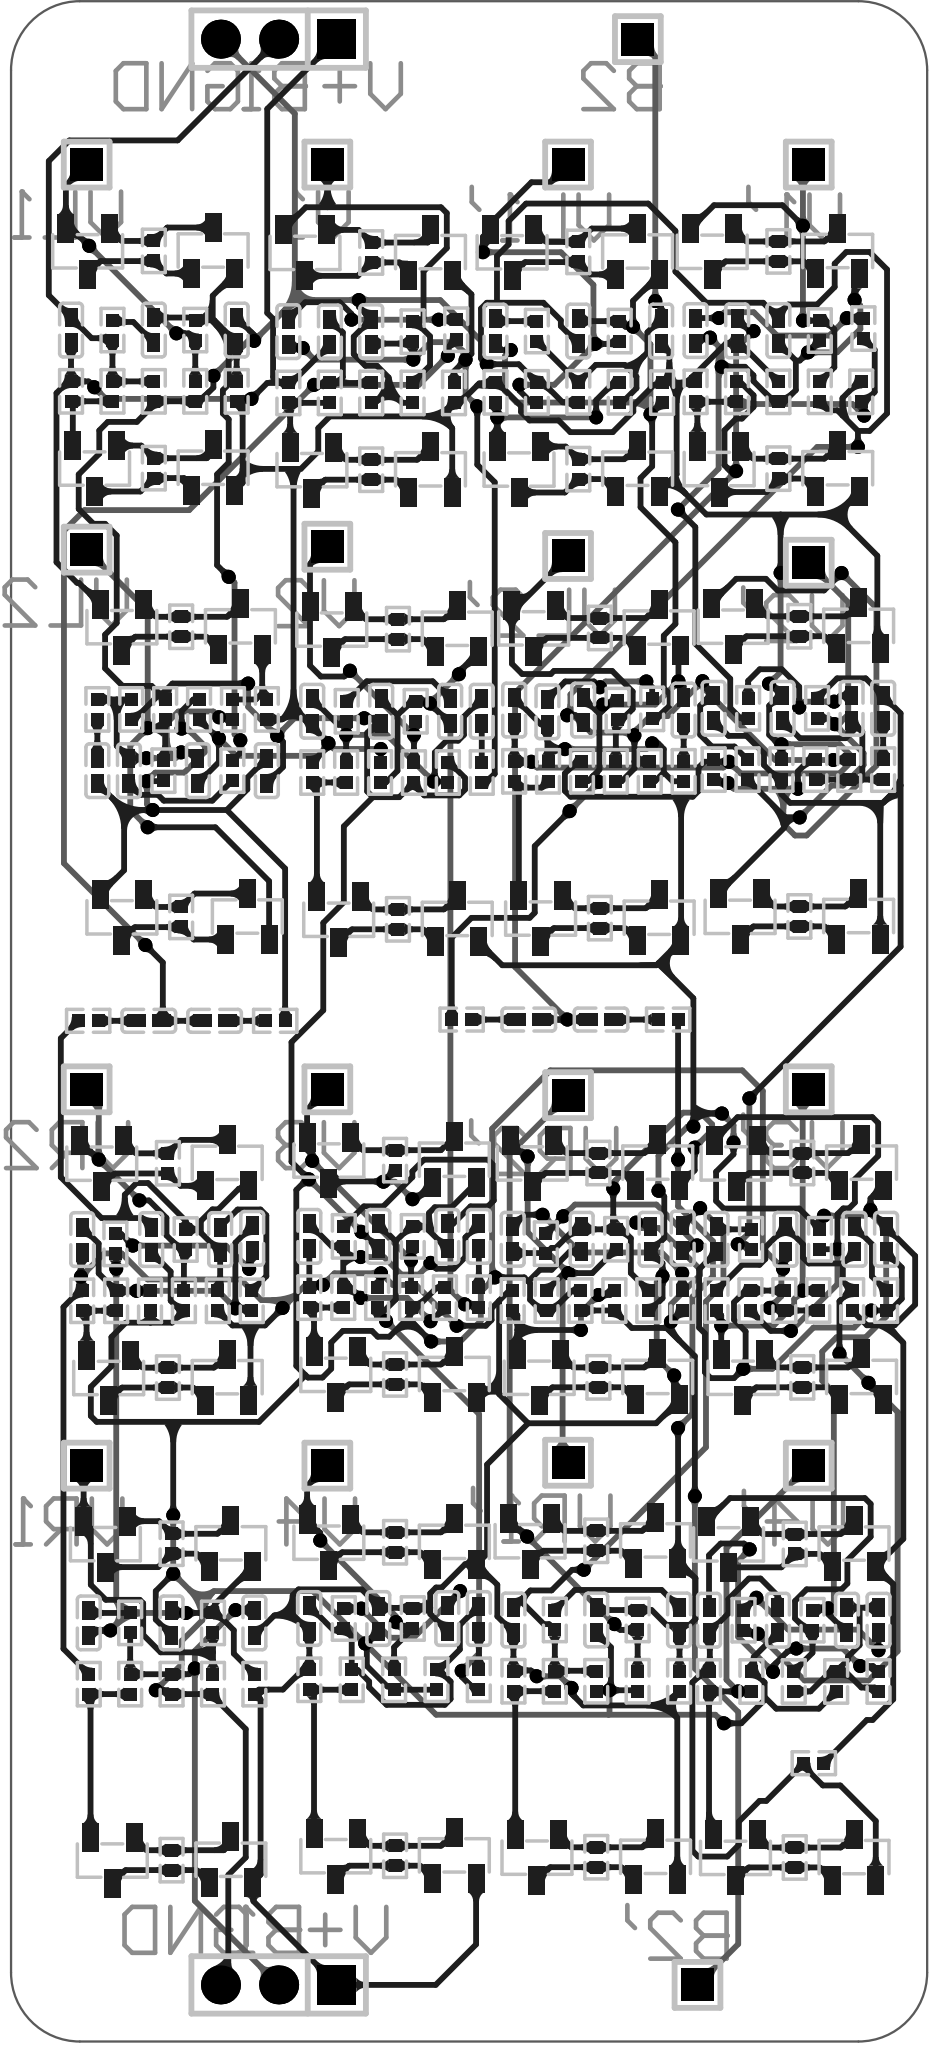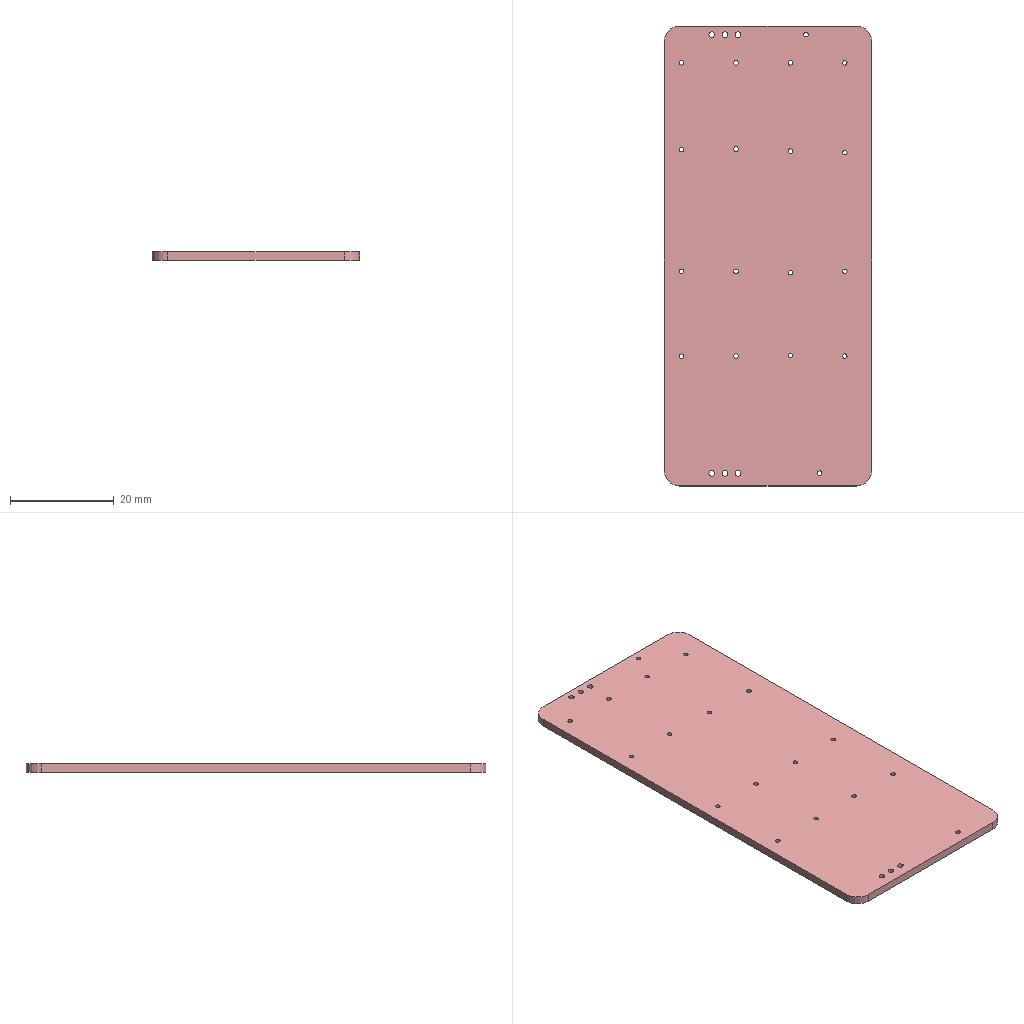Circuit board layout | Altium Designer | box 40 x 88.8 x 1.6 mm
Layer stack:
# Altium Designer layer stack of  (unit mm; dielectric type: 0 none, 1 core, 2 prepreg, 3 surface material)
index,name,kind,layer,copper_thickness_mm,dielectric_type,dielectric_thickness_mm,dielectric_material,dielectric_constant
0,Top Paste Mask Layer,other,,,,,,
1,Top Silkscreen Layer,other,,,,,,
2,Top Solder Mask Layer,dielectric,,,3,0.01,,3.3
3,Top Layer,copper,Top Layer,0.035,,,,
4,Dielectric1,dielectric,,,3,1.51,FR4,4.5
5,Bottom Layer,copper,Bottom Layer,0.035,,,,
6,Bottom Solder Mask Layer,dielectric,,,3,0.01,,3.3
7,Bottom Silkscreen Layer,other,,,,,,
8,Bottom Paste Mask Layer,other,,,,,,
# drill layer pairs: low layer,high layer
drill_pair,Top Layer,Bottom Layer
Part placement:
Designator,Comment,Layer,Footprint,Center-X(mm),Center-Y(mm),Rotation
C2,0.1uF,TopLayer,C0402,82.435,150.707,270
C4,0.1uF,TopLayer,C0402,78.819,150.707,90
C5,0.1uF,TopLayer,C0402,86.051,150.707,90
Q1,MMBT3906,TopLayer,SOT-23-3_L2.9-W1.3-P1.90-LS2.4-BR,85.023,154.171,270
Q2,MMBT3904,TopLayer,SOT-23-3_L2.9-W1.3-P1.90-LS2.4-BR,79.847,144.678,90
Q3,MMBT3906,TopLayer,SOT-23-3_L2.9-W1.3-P1.90-LS2.4-BR,85.023,144.713,270
Q4,MMBT3904,TopLayer,SOT-23-3_L2.9-W1.3-P1.90-LS2.4-BR,79.544,154.136,90
R1,1,TopLayer,R0402,80.627,150.707,270
R3,2.2K,TopLayer,R0402,82.435,148.04,270
R4,2.2K,TopLayer,R0402,86.051,148.04,90
Rb1,1K,TopLayer,R0402,82.435,144.696,270
Rb2,1K,TopLayer,R0402,82.435,154.153,270
Rp1,200K,TopLayer,R0402,78.819,148.04,270
Rp2,200K,TopLayer,R0402,84.243,150.707,270
Rs1,200,TopLayer,R0402,80.627,148.04,90
Rs2,200,TopLayer,R0402,84.243,148.04,270
Rb3,1K,TopLayer,R0402,83.627,137.791,90
Q6,MMBT3906,TopLayer,SOT-23-3_L2.9-W1.3-P1.90-LS2.4-BR,81.039,137.773,90
Q5,MMBT3904,TopLayer,SOT-23-3_L2.9-W1.3-P1.90-LS2.4-BR,86.215,137.808,270
R7,2.2K,TopLayer,R0402,81.448,134.193,270
Rp3,200K,TopLayer,R0402,87.37,134.193,90
Rs3,200,TopLayer,R0402,85.889,134.193,270
R9,2.2K,TopLayer,R0402,84.409,134.193,90
Rs4,200,TopLayer,R0402,82.929,134.193,90
C1,0.1uF,TopLayer,C0402,81.347,131.526,270
C6,0.1uF,TopLayer,C0402,84.358,131.526,90
Rp4,200K,TopLayer,R0402,82.852,131.526,90
R5,1,TopLayer,R0402,85.864,131.526,90
C7,0.1uF,TopLayer,C0402,87.37,131.526,270
Q7,MMBT3904,TopLayer,SOT-23-3_L2.9-W1.3-P1.90-LS2.4-BR,86.517,125.176,270
Rb4,1K,TopLayer,R0402,83.627,125.158,90
Q8,MMBT3906,TopLayer,SOT-23-3_L2.9-W1.3-P1.90-LS2.4-BR,81.039,125.141,90
C8,0.1uF,TopLayer,C0402,79.968,131.526,90
H1,,TopLayer,HDR-TH_3P-P2.54-V-M,87.884,163.373,180
C9,0.02uF,TopLayer,C0402,85.087,120.635,0
C17,0.02uF,TopLayer,C0402,82.215,120.635,180
R6,1,TopLayer,R0402,79.968,134.193,90
R10,1,TopLayer,R0402,87.734,120.635,0
R18,1,TopLayer,R0402,79.568,120.635,180
Rp7,200K,TopLayer,R0402,79.307,108.447,270
Rs7,200,TopLayer,R0402,80.787,108.447,90
R16,2.2K,TopLayer,R0402,82.268,108.447,270
Rs8,200,TopLayer,R0402,83.748,108.447,270
R17,2.2K,TopLayer,R0402,85.228,108.447,90
R15,1,TopLayer,R0402,86.709,108.447,270
C14,0.1uF,TopLayer,C0402,79.307,111.114,90
R19,1,TopLayer,R0402,95.635,150.725,270
C15,0.1uF,TopLayer,C0402,82.319,111.114,270
Rp8,200K,TopLayer,R0402,83.824,111.114,270
C16,0.1uF,TopLayer,C0402,85.33,111.114,90
C18,0.1uF,TopLayer,C0402,90.123,150.626,90
Rb7,1K,TopLayer,R0402,83.05,105.103,270
Q13,MMBT3904,TopLayer,SOT-23-3_L2.9-W1.3-P1.90-LS2.4-BR,80.462,105.085,90
Q14,MMBT3906,TopLayer,SOT-23-3_L2.9-W1.3-P1.90-LS2.4-BR,85.638,105.121,270
Q16,MMBT3906,TopLayer,SOT-23-3_L2.9-W1.3-P1.90-LS2.4-BR,85.638,114.451,270
Q15,MMBT3904,TopLayer,SOT-23-3_L2.9-W1.3-P1.90-LS2.4-BR,80.159,114.416,90
Rb8,1K,TopLayer,R0402,83.05,114.434,270
Rb5,1K,TopLayer,R0402,83.209,84.095,270
Q10,MMBT3906,TopLayer,SOT-23-3_L2.9-W1.3-P1.90-LS2.4-BR,85.797,84.113,270
Q9,MMBT3904,TopLayer,SOT-23-3_L2.9-W1.3-P1.90-LS2.4-BR,80.621,84.078,90
R13,2.2K,TopLayer,R0402,86.825,91.757,90
Rp5,200K,TopLayer,R0402,79.593,91.757,270
Rs5,200,TopLayer,R0402,81.401,91.757,90
R14,2.2K,TopLayer,R0402,83.209,91.757,270
Rs6,200,TopLayer,R0402,85.017,91.757,270
Rp6,200K,TopLayer,R0402,85.017,94.424,270
R11,1,TopLayer,R0402,81.401,94.424,270
C10,0.1uF,TopLayer,C0402,86.825,94.424,90
C11,0.1uF,TopLayer,C0402,83.209,94.424,270
C12,0.1uF,TopLayer,C0402,79.593,94.424,90
Q11,MMBT3904,TopLayer,SOT-23-3_L2.9-W1.3-P1.90-LS2.4-BR,80.319,97.853,90
Rb6,1K,TopLayer,R0402,83.209,97.871,270
Q12,MMBT3906,TopLayer,SOT-23-3_L2.9-W1.3-P1.90-LS2.4-BR,85.797,97.888,270
Rb9,1K,TopLayer,R0402,91.925,144.627,270
Q18,MMBT3906,TopLayer,SOT-23-3_L2.9-W1.3-P1.90-LS2.4-BR,94.513,144.644,270
Q17,MMBT3904,TopLayer,SOT-23-3_L2.9-W1.3-P1.90-LS2.4-BR,89.337,144.609,90
R20,2.2K,TopLayer,R0402,95.541,147.971,90
Rp9,200K,TopLayer,R0402,88.309,147.971,270
Rs9,200,TopLayer,R0402,90.117,147.971,90
R21,2.55K,TopLayer,R0402,91.925,147.971,270
Rs10,200,TopLayer,R0402,93.733,147.971,270
Rp10,200K,TopLayer,R0402,93.733,150.638,90
R12,1,TopLayer,R0402,80.756,110.924,270
C13,0.1uF,TopLayer,C0402,86.73,111.165,270
C19,0.1uF,TopLayer,C0402,91.925,150.638,90
C20,0.1uF,TopLayer,C0402,88.309,150.638,90
Q19,MMBT3904,TopLayer,SOT-23-3_L2.9-W1.3-P1.90-LS2.4-BR,89.034,154.067,90
Rb10,1K,TopLayer,R0402,91.925,154.084,270
Q20,MMBT3906,TopLayer,SOT-23-3_L2.9-W1.3-P1.90-LS2.4-BR,94.513,154.102,270
Rb11,1K,TopLayer,R0402,93.094,125.053,270
Q21,MMBT3904,TopLayer,SOT-23-3_L2.9-W1.3-P1.90-LS2.4-BR,90.505,125.035,90
Q22,MMBT3906,TopLayer,SOT-23-3_L2.9-W1.3-P1.90-LS2.4-BR,95.682,125.07,270
Rs11,200,TopLayer,R0402,90.831,131.445,90
R24,2.2K,TopLayer,R0402,95.272,131.445,90
R22,1,TopLayer,R0402,96.752,131.445,270
Rp11,200K,TopLayer,R0402,89.351,131.445,270
Rs12,200,TopLayer,R0402,93.792,131.445,270
R25,2.2K,TopLayer,R0402,92.312,131.445,270
C21,0.1uF,TopLayer,C0402,96.752,134.112,270
C22,0.1uF,TopLayer,C0402,89.351,134.112,90
R23,1,TopLayer,R0402,90.857,134.112,270
C23,0.1uF,TopLayer,C0402,92.362,134.112,270
C24,0.1uF,TopLayer,C0402,95.374,134.112,90
Rp12,200K,TopLayer,R0402,93.868,134.112,270
Rb12,1K,TopLayer,R0402,93.094,137.685,270
Q23,MMBT3904,TopLayer,SOT-23-3_L2.9-W1.3-P1.90-LS2.4-BR,90.203,137.668,90
Q24,MMBT3906,TopLayer,SOT-23-3_L2.9-W1.3-P1.90-LS2.4-BR,95.682,137.703,270
Rb13,1K,TopLayer,R0402,92.967,105.241,270
Q25,MMBT3904,TopLayer,SOT-23-3_L2.9-W1.3-P1.90-LS2.4-BR,90.379,105.223,90
Q26,MMBT3906,TopLayer,SOT-23-3_L2.9-W1.3-P1.90-LS2.4-BR,95.555,105.258,270
Rs13,200,TopLayer,R0402,90.704,108.585,90
R28,2.2K,TopLayer,R0402,95.145,108.585,90
R26,1,TopLayer,R0402,96.626,108.585,270
Rp13,200K,TopLayer,R0402,89.224,108.585,270
Rs14,200,TopLayer,R0402,93.665,108.585,270
R29,2.2K,TopLayer,R0402,92.185,108.585,270
C25,0.1uF,TopLayer,C0402,96.626,111.252,270
C26,0.1uF,TopLayer,C0402,89.224,111.252,90
R27,1,TopLayer,R0402,90.73,111.252,270
C27,0.1uF,TopLayer,C0402,92.235,111.252,270
C28,0.1uF,TopLayer,C0402,95.247,111.252,90
Rp14,200K,TopLayer,R0402,93.741,111.252,270
Rb14,1K,TopLayer,R0402,92.967,114.571,270
Q27,MMBT3904,TopLayer,SOT-23-3_L2.9-W1.3-P1.90-LS2.4-BR,90.076,114.554,90
Q28,MMBT3906,TopLayer,SOT-23-3_L2.9-W1.3-P1.90-LS2.4-BR,95.555,114.589,270
Rb15,1K,TopLayer,R0402,92.967,84.286,270
Q29,MMBT3904,TopLayer,SOT-23-3_L2.9-W1.3-P1.90-LS2.4-BR,90.379,84.268,90
Q30,MMBT3906,TopLayer,SOT-23-3_L2.9-W1.3-P1.90-LS2.4-BR,95.555,84.303,270
Rs15,200,TopLayer,R0402,91.074,91.948,90
R32,2.2K,TopLayer,R0402,94.775,91.948,270
R30,1,TopLayer,R0402,96.626,91.948,270
Rp15,200K,TopLayer,R0402,89.224,91.948,270
Rs16,200,TopLayer,R0402,92.925,91.948,270
R35,2.2K,TopLayer,R0402,104.626,147.984,270
C29,0.1uF,TopLayer,C0402,96.626,94.615,270
C30,0.1uF,TopLayer,C0402,89.224,94.615,90
R31,1,TopLayer,R0402,90.73,94.615,270
C31,0.1uF,TopLayer,C0402,92.235,94.615,270
C32,0.1uF,TopLayer,C0402,95.247,94.615,90
Rp16,200K,TopLayer,R0402,93.741,94.615,270
Rb16,1K,TopLayer,R0402,92.967,97.934,270
Q31,MMBT3904,TopLayer,SOT-23-3_L2.9-W1.3-P1.90-LS2.4-BR,90.076,97.917,90
Q32,MMBT3906,TopLayer,SOT-23-3_L2.9-W1.3-P1.90-LS2.4-BR,95.555,97.952,270
Q33,MMBT3904,TopLayer,SOT-23-3_L2.9-W1.3-P1.90-LS2.4-BR,98.379,144.635,90
Q34,MMBT3906,TopLayer,SOT-23-3_L2.9-W1.3-P1.90-LS2.4-BR,103.556,144.67,270
Rb17,1K,TopLayer,R0402,100.968,144.653,270
R36,2.2K,TopLayer,R0402,100.968,147.997,270
Rs17,200,TopLayer,R0402,102.776,147.997,270
Rp17,200K,TopLayer,R0402,97.352,147.997,270
Rs18,200,TopLayer,R0402,99.16,147.997,90
Rp18,200K,TopLayer,R0402,102.776,150.664,270
R33,1,TopLayer,R0402,99.16,150.664,270
C33,0.1uF,TopLayer,C0402,104.584,150.664,90
C34,0.1uF,TopLayer,C0402,100.968,150.664,270
C35,0.1uF,TopLayer,C0402,97.352,150.664,90
Q36,MMBT3906,TopLayer,SOT-23-3_L2.9-W1.3-P1.90-LS2.4-BR,103.556,154.128,270
Rb18,1K,TopLayer,R0402,100.968,154.11,270
Q35,MMBT3904,TopLayer,SOT-23-3_L2.9-W1.3-P1.90-LS2.4-BR,98.077,154.093,90
Rb19,1K,TopLayer,R0402,101.909,125.106,270
Q37,MMBT3904,TopLayer,SOT-23-3_L2.9-W1.3-P1.90-LS2.4-BR,99.321,125.088,90
Q38,MMBT3906,TopLayer,SOT-23-3_L2.9-W1.3-P1.90-LS2.4-BR,104.498,125.123,270
R34,1,TopLayer,R0402,104.193,134.216,270
C36,0.1uF,TopLayer,C0402,99.621,134.089,90
R38,2.2K,TopLayer,R0402,104.088,131.498,90
Rs19,200,TopLayer,R0402,99.647,131.498,90
R37,1,TopLayer,R0402,105.568,131.498,270
Rp19,200K,TopLayer,R0402,98.167,131.498,270
Rs20,200,TopLayer,R0402,102.608,131.498,270
R39,2.2K,TopLayer,R0402,101.127,131.498,270
C37,0.1uF,TopLayer,C0402,98.167,134.165,90
R40,1,TopLayer,R0402,95.874,120.69,180
C38,0.1uF,TopLayer,C0402,101.178,134.165,270
C39,0.1uF,TopLayer,C0402,105.568,134.165,270
C40,0.02uF,TopLayer,C0402,98.805,120.69,180
Rp20,200K,TopLayer,R0402,102.684,134.165,270
Rb20,1K,TopLayer,R0402,101.909,137.738,270
Q39,MMBT3904,TopLayer,SOT-23-3_L2.9-W1.3-P1.90-LS2.4-BR,99.019,137.72,90
Q40,MMBT3906,TopLayer,SOT-23-3_L2.9-W1.3-P1.90-LS2.4-BR,104.498,137.756,270
C48,0.02uF,TopLayer,C0402,101.96,120.69,0
R48,1,TopLayer,R0402,104.891,120.69,0
Rb21,1K,TopLayer,R0402,101.846,105.114,270
Q41,MMBT3904,TopLayer,SOT-23-3_L2.9-W1.3-P1.90-LS2.4-BR,99.258,105.096,90
Q42,MMBT3906,TopLayer,SOT-23-3_L2.9-W1.3-P1.90-LS2.4-BR,104.434,105.131,270
R43,2.2K,TopLayer,R0402,104.025,108.458,90
Rs21,200,TopLayer,R0402,102.544,108.458,270
R44,2.2K,TopLayer,R0402,101.064,108.458,90
R41,1,TopLayer,R0402,105.505,108.458,270
Rs22,200,TopLayer,R0402,99.584,108.458,270
Rp21,200K,TopLayer,R0402,98.103,108.458,270
R42,1,TopLayer,R0402,99.552,110.934,270
C41,0.1uF,TopLayer,C0402,104.126,111.125,90
Rp22,200K,TopLayer,R0402,102.62,111.125,270
C42,0.1uF,TopLayer,C0402,101.115,111.125,270
C43,0.1uF,TopLayer,C0402,98.103,111.125,90
C44,0.1uF,TopLayer,C0402,105.526,111.176,270
Rb22,1K,TopLayer,R0402,101.846,114.444,270
Q44,MMBT3906,TopLayer,SOT-23-3_L2.9-W1.3-P1.90-LS2.4-BR,104.434,114.462,270
Q43,MMBT3904,TopLayer,SOT-23-3_L2.9-W1.3-P1.90-LS2.4-BR,98.955,114.427,90
Rb23,1K,TopLayer,R0402,101.751,84.222,270
Q45,MMBT3904,TopLayer,SOT-23-3_L2.9-W1.3-P1.90-LS2.4-BR,99.163,84.205,90
Q46,MMBT3906,TopLayer,SOT-23-3_L2.9-W1.3-P1.90-LS2.4-BR,104.339,84.24,270
Rs23,200,TopLayer,R0402,99.943,91.884,90
Rp23,200K,TopLayer,R0402,98.135,91.884,270
R46,2.2K,TopLayer,R0402,101.751,91.884,270
Rs24,200,TopLayer,R0402,103.559,91.884,270
R47,2.2K,TopLayer,R0402,105.367,91.884,90
C45,0.1uF,TopLayer,C0402,98.135,94.551,90
C46,0.1uF,TopLayer,C0402,101.751,94.551,270
R45,1,TopLayer,R0402,99.943,94.551,270
C47,0.1uF,TopLayer,C0402,105.367,94.551,90
Rp24,200K,TopLayer,R0402,103.559,94.551,270
Rb24,1K,TopLayer,R0402,101.751,97.998,270
Q48,MMBT3906,TopLayer,SOT-23-3_L2.9-W1.3-P1.90-LS2.4-BR,104.339,98.015,270
Q47,MMBT3904,TopLayer,SOT-23-3_L2.9-W1.3-P1.90-LS2.4-BR,98.861,97.98,90
Rb25,1K,TopLayer,R0402,109.705,144.674,270
Q49,MMBT3904,TopLayer,SOT-23-3_L2.9-W1.3-P1.90-LS2.4-BR,107.117,144.657,90
Q50,MMBT3906,TopLayer,SOT-23-3_L2.9-W1.3-P1.90-LS2.4-BR,112.293,144.692,270
Rs25,200,TopLayer,R0402,107.897,148.018,90
Rp25,200K,TopLayer,R0402,106.089,148.018,270
Rs26,200,TopLayer,R0402,111.513,148.018,270
R50,2.2K,TopLayer,R0402,109.705,148.018,270
R51,2.55K,TopLayer,R0402,113.321,148.018,90
C49,0.1uF,TopLayer,C0402,107.903,150.673,90
C50,0.1uF,TopLayer,C0402,109.705,150.685,90
C51,0.1uF,TopLayer,C0402,106.089,150.685,90
Rp26,200K,TopLayer,R0402,111.513,150.685,90
R49,1,TopLayer,R0402,113.415,150.772,270
Rb26,1K,TopLayer,R0402,109.705,154.132,270
Q52,MMBT3906,TopLayer,SOT-23-3_L2.9-W1.3-P1.90-LS2.4-BR,112.293,154.149,270
Q51,MMBT3904,TopLayer,SOT-23-3_L2.9-W1.3-P1.90-LS2.4-BR,106.814,154.114,90
Rs27,200,TopLayer,R0402,111.318,131.572,270
Rp27,200K,TopLayer,R0402,106.877,131.572,270
C52,0.1uF,TopLayer,C0402,112.9,134.239,90
Rp28,200K,TopLayer,R0402,111.394,134.239,270
C53,0.1uF,TopLayer,C0402,109.888,134.239,270
R52,1,TopLayer,R0402,108.383,134.239,270
C54,0.1uF,TopLayer,C0402,106.877,134.239,90
C55,0.1uF,TopLayer,C0402,114.278,134.239,270
Rb27,1K,TopLayer,R0402,110.62,137.812,270
Q54,MMBT3906,TopLayer,SOT-23-3_L2.9-W1.3-P1.90-LS2.4-BR,113.208,137.83,270
Q53,MMBT3904,TopLayer,SOT-23-3_L2.9-W1.3-P1.90-LS2.4-BR,107.729,137.795,90
Rb28,1K,TopLayer,R0402,110.62,125.18,270
Q56,MMBT3906,TopLayer,SOT-23-3_L2.9-W1.3-P1.90-LS2.4-BR,113.208,125.197,270
Q55,MMBT3904,TopLayer,SOT-23-3_L2.9-W1.3-P1.90-LS2.4-BR,108.031,125.162,90
Rs28,200,TopLayer,R0402,108.357,131.572,90
R53,1,TopLayer,R0402,114.278,131.572,270
R54,2.2K,TopLayer,R0402,112.798,131.572,90
R55,2.2K,TopLayer,R0402,109.838,131.572,270
R56,1,TopLayer,R0402,108.51,111.125,270
C56,0.1uF,TopLayer,C0402,107.004,111.125,90
C57,0.1uF,TopLayer,C0402,114.406,111.125,270
C58,0.1uF,TopLayer,C0402,110.015,111.125,270
C59,0.1uF,TopLayer,C0402,113.027,111.125,90
Rp29,200K,TopLayer,R0402,111.521,111.125,270
Rb29,1K,TopLayer,R0402,110.747,114.444,270
Q58,MMBT3906,TopLayer,SOT-23-3_L2.9-W1.3-P1.90-LS2.4-BR,113.335,114.462,270
Q57,MMBT3904,TopLayer,SOT-23-3_L2.9-W1.3-P1.90-LS2.4-BR,107.856,114.427,90
Rb30,1K,TopLayer,R0402,110.747,105.114,270
Q59,MMBT3904,TopLayer,SOT-23-3_L2.9-W1.3-P1.90-LS2.4-BR,108.159,105.096,90
Q60,MMBT3906,TopLayer,SOT-23-3_L2.9-W1.3-P1.90-LS2.4-BR,113.335,105.131,270
R58,2.2K,TopLayer,R0402,109.965,108.458,270
Rs29,200,TopLayer,R0402,108.484,108.458,90
R59,2.2K,TopLayer,R0402,112.925,108.458,90
Rs30,200,TopLayer,R0402,111.445,108.458,270
Rp30,200K,TopLayer,R0402,107.004,108.458,270
R57,1,TopLayer,R0402,114.406,108.458,270
C60,0.1uF,TopLayer,C0402,114.077,94.54,270
C61,0.1uF,TopLayer,C0402,112.699,94.54,90
C62,0.1uF,TopLayer,C0402,109.687,94.54,270
R60,1,TopLayer,R0402,108.181,94.54,270
Rp31,200K,TopLayer,R0402,111.193,94.54,270
C63,0.1uF,TopLayer,C0402,106.676,94.54,90
Rb31,1K,TopLayer,R0402,110.418,97.86,270
Q62,MMBT3906,TopLayer,SOT-23-3_L2.9-W1.3-P1.90-LS2.4-BR,113.007,97.878,270
Q61,MMBT3904,TopLayer,SOT-23-3_L2.9-W1.3-P1.90-LS2.4-BR,107.528,97.843,90
Rb32,1K,TopLayer,R0402,110.418,84.212,270
Q63,MMBT3904,TopLayer,SOT-23-3_L2.9-W1.3-P1.90-LS2.4-BR,107.83,84.194,90
Q64,MMBT3906,TopLayer,SOT-23-3_L2.9-W1.3-P1.90-LS2.4-BR,113.007,84.229,270
R62,2.2K,TopLayer,R0402,112.227,91.874,270
R61,1,TopLayer,R0402,114.077,91.874,270
Rp32,200K,TopLayer,R0402,106.676,91.874,270
Rs31,200,TopLayer,R0402,110.376,91.874,270
Rs32,200,TopLayer,R0402,108.526,91.874,90
H2,,TopLayer,HDR-TH_1P-V-M_XKB_X4611WV-01I-C28D40,79.502,157.912,0
H3,,TopLayer,HDR-TH_1P-V-M_XKB_X4611WV-01I-C28D40,79.502,141.148,0
H4,,TopLayer,HDR-TH_1P-V-M_XKB_X4611WV-01I-C28D40,79.502,117.653,0
H5,,TopLayer,HDR-TH_1P-V-M_XKB_X4611WV-01I-C28D40,79.502,101.27,0
H6,,TopLayer,HDR-TH_1P-V-M_XKB_X4611WV-01I-C28D40,90.011,157.912,0
H7,,TopLayer,HDR-TH_1P-V-M_XKB_X4611WV-01I-C28D40,90.011,141.275,0
H9,,TopLayer,HDR-TH_1P-V-M_XKB_X4611WV-01I-C28D40,90.011,117.653,0
H10,,TopLayer,HDR-TH_1P-V-M_XKB_X4611WV-01I-C28D40,90.011,101.27,0
H12,,TopLayer,HDR-TH_1P-V-M_XKB_X4611WV-01I-C28D40,100.52,157.912,0
H13,,TopLayer,HDR-TH_1P-V-M_XKB_X4611WV-01I-C28D40,100.52,140.872,0
H14,,TopLayer,HDR-TH_1P-V-M_XKB_X4611WV-01I-C28D40,100.52,117.399,0
H15,,TopLayer,HDR-TH_1P-V-M_XKB_X4611WV-01I-C28D40,100.52,101.397,0
H16,,TopLayer,HDR-TH_1P-V-M_XKB_X4611WV-01I-C28D40,111.03,157.912,0
H17,,TopLayer,HDR-TH_1P-V-M_XKB_X4611WV-01I-C28D40,111.03,140.578,0
H18,,TopLayer,HDR-TH_1P-V-M_XKB_X4611WV-01I-C28D40,111.03,117.653,0
H19,,TopLayer,HDR-TH_1P-V-M_XKB_X4611WV-01I-C28D40,111.03,101.27,0
H20,,TopLayer,HDR-TH_1P-V-M_XKB_X4611WV-01I-C28D40,103.569,163.373,0
H21,,TopLayer,HDR-TH_3P-P2.54-V-M,87.884,78.664,180
H22,,TopLayer,HDR-TH_1P-V-M_XKB_X4611WV-01I-C28D40,106.172,78.664,0
R63,2.2K,TopLayer,R0402,111.252,88.316,180
Pad and via stacks:
# Altium Designer via and pad stacks of  (unit mm). Each distinct definition once, with the count of objects using it.
# via: kind,start_layer,end_layer,hole_mm,diameter_mm,mode(0 simple;1 top-mid-bottom;2 full stack),diameter_per_layer,count,example_net
# pad: kind,layer,hole_mm,hole_type(0 round;1 square;2 slot),plating,top_size,top_shape(1 round;2 rect;3 octagon;9 rounded rect),mid_size,bottom_size,mode,footprint,size_per_layer,count,example
pad,Top Layer,0,0,plated,0.7901x0.54,2,0.7901x0.54,0.7901x0.54,0,C0402,,124,C2.2
pad,Top Layer,0,0,plated,1.25x0.7,2,1.25x0.7,1.25x0.7,0,SOT-23-3_L2.9-W1.3-P1.90-LS2.4-BR,,192,Q1.1
pad,Top Layer,0,0,plated,0.5657x0.54,2,0.5657x0.54,0.5657x0.54,0,R0402,,314,R1.2
pad,Multi-Layer,1.1,0,plated,1.7x1.7,2,1.7x1.7,1.7x1.7,0,HDR-TH_3P-P2.54-V-M,,2,H1.1
pad,Multi-Layer,1.1,0,plated,1.7x1.7,1,1.7x1.7,1.7x1.7,0,HDR-TH_3P-P2.54-V-M,,4,H1.2
pad,Multi-Layer,0.9,0,plated,1.4x1.4,2,1.4x1.4,1.4x1.4,0,HDR-TH_1P-V-M_XKB_X4611WV-01I-C28D40,,18,H2.1
via,Top Layer,Bottom Layer,0.3048,0.61,0,,177,$1N1020